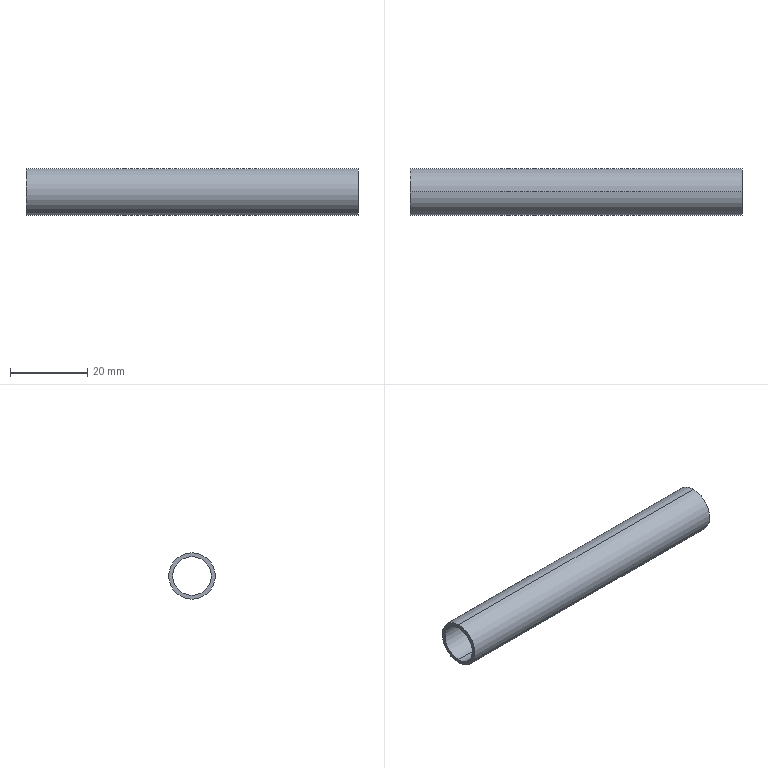Part | SolidWorks | features 3DProfileFeature 2, Sweep 1 | 1 solid | 6 faces | box 85.757 x 12 x 12 mm | volume 2964 mm3 | cylinder 4 | plane 2 | commonest cylinder face diameters 10 x2 12 x2
STEP:
#1=CARTESIAN_POINT('',(860.166,1814.095,417.913));
#2=VERTEX_POINT('',#1);
#3=CARTESIAN_POINT('',(860.166,1814.095,427.913));
#4=VERTEX_POINT('',#3);
#5=CARTESIAN_POINT('',(860.166,1814.095,422.913));
#6=DIRECTION('',(-1.,0.,0.));
#7=DIRECTION('',(0.,0.,1.));
#8=AXIS2_PLACEMENT_3D('',#5,#6,#7);
#9=CIRCLE('',#8,5.);
#10=EDGE_CURVE('',#2,#4,#9,.T.);
#11=ORIENTED_EDGE('',*,*,#10,.F.);
#12=CARTESIAN_POINT('',(774.41,1814.095,417.913));
#13=VERTEX_POINT('',#12);
#14=CARTESIAN_POINT('',(860.166,1814.095,417.913));
#15=DIRECTION('',(-1.,0.,0.));
#16=VECTOR('',#15,1000.);
#17=LINE('',#14,#16);
#18=EDGE_CURVE('',#2,#13,#17,.T.);
#19=ORIENTED_EDGE('',*,*,#18,.T.);
#20=CARTESIAN_POINT('',(774.41,1814.095,427.913));
#21=VERTEX_POINT('',#20);
#22=CARTESIAN_POINT('',(774.41,1814.095,422.913));
#23=DIRECTION('',(-1.,0.,0.));
#24=DIRECTION('',(0.,0.,1.));
#25=AXIS2_PLACEMENT_3D('',#22,#23,#24);
#26=CIRCLE('',#25,5.);
#27=EDGE_CURVE('',#13,#21,#26,.T.);
#28=ORIENTED_EDGE('',*,*,#27,.T.);
#29=CARTESIAN_POINT('',(860.166,1814.095,427.913));
#30=DIRECTION('',(-1.,0.,0.));
#31=VECTOR('',#30,1000.);
#32=LINE('',#29,#31);
#33=EDGE_CURVE('',#4,#21,#32,.T.);
#34=ORIENTED_EDGE('',*,*,#33,.F.);
#35=EDGE_LOOP('',(#11,#19,#28,#34));
#36=FACE_OUTER_BOUND('',#35,.T.);
#37=CARTESIAN_POINT('',(860.166,1814.095,422.913));
#38=DIRECTION('',(-1.,0.,0.));
#39=DIRECTION('',(0.,0.,1.));
#40=AXIS2_PLACEMENT_3D('',#37,#38,#39);
#41=CYLINDRICAL_SURFACE('',#40,5.);
#42=ADVANCED_FACE('',(#36),#41,.F.);
#43=CARTESIAN_POINT('',(860.166,1814.095,428.913));
#44=VERTEX_POINT('',#43);
#45=CARTESIAN_POINT('',(860.166,1814.095,416.913));
#46=VERTEX_POINT('',#45);
#47=CARTESIAN_POINT('',(860.166,1814.095,422.913));
#48=DIRECTION('',(-1.,0.,0.));
#49=DIRECTION('',(0.,0.,1.));
#50=AXIS2_PLACEMENT_3D('',#47,#48,#49);
#51=CIRCLE('',#50,6.);
#52=EDGE_CURVE('',#44,#46,#51,.T.);
#53=ORIENTED_EDGE('',*,*,#52,.T.);
#54=CARTESIAN_POINT('',(774.41,1814.095,416.913));
#55=VERTEX_POINT('',#54);
#56=CARTESIAN_POINT('',(860.166,1814.095,416.913));
#57=DIRECTION('',(-1.,0.,0.));
#58=VECTOR('',#57,1000.);
#59=LINE('',#56,#58);
#60=EDGE_CURVE('',#46,#55,#59,.T.);
#61=ORIENTED_EDGE('',*,*,#60,.T.);
#62=CARTESIAN_POINT('',(774.41,1814.095,428.913));
#63=VERTEX_POINT('',#62);
#64=CARTESIAN_POINT('',(774.41,1814.095,422.913));
#65=DIRECTION('',(-1.,0.,0.));
#66=DIRECTION('',(0.,0.,1.));
#67=AXIS2_PLACEMENT_3D('',#64,#65,#66);
#68=CIRCLE('',#67,6.);
#69=EDGE_CURVE('',#63,#55,#68,.T.);
#70=ORIENTED_EDGE('',*,*,#69,.F.);
#71=CARTESIAN_POINT('',(860.166,1814.095,428.913));
#72=DIRECTION('',(-1.,0.,0.));
#73=VECTOR('',#72,1000.);
#74=LINE('',#71,#73);
#75=EDGE_CURVE('',#44,#63,#74,.T.);
#76=ORIENTED_EDGE('',*,*,#75,.F.);
#77=EDGE_LOOP('',(#53,#61,#70,#76));
#78=FACE_OUTER_BOUND('',#77,.T.);
#79=CARTESIAN_POINT('',(860.166,1814.095,422.913));
#80=DIRECTION('',(-1.,0.,0.));
#81=DIRECTION('',(0.,0.,1.));
#82=AXIS2_PLACEMENT_3D('',#79,#80,#81);
#83=CYLINDRICAL_SURFACE('',#82,6.);
#84=ADVANCED_FACE('',(#78),#83,.T.);
#85=ORIENTED_EDGE('',*,*,#60,.F.);
#86=CARTESIAN_POINT('',(860.166,1814.095,422.913));
#87=DIRECTION('',(-1.,0.,0.));
#88=DIRECTION('',(0.,0.,1.));
#89=AXIS2_PLACEMENT_3D('',#86,#87,#88);
#90=CIRCLE('',#89,6.);
#91=EDGE_CURVE('',#46,#44,#90,.T.);
#92=ORIENTED_EDGE('',*,*,#91,.T.);
#93=ORIENTED_EDGE('',*,*,#75,.T.);
#94=CARTESIAN_POINT('',(774.41,1814.095,422.913));
#95=DIRECTION('',(-1.,0.,0.));
#96=DIRECTION('',(0.,0.,1.));
#97=AXIS2_PLACEMENT_3D('',#94,#95,#96);
#98=CIRCLE('',#97,6.);
#99=EDGE_CURVE('',#55,#63,#98,.T.);
#100=ORIENTED_EDGE('',*,*,#99,.F.);
#101=EDGE_LOOP('',(#85,#92,#93,#100));
#102=FACE_OUTER_BOUND('',#101,.T.);
#103=CARTESIAN_POINT('',(860.166,1814.095,422.913));
#104=DIRECTION('',(-1.,0.,0.));
#105=DIRECTION('',(0.,0.,1.));
#106=AXIS2_PLACEMENT_3D('',#103,#104,#105);
#107=CYLINDRICAL_SURFACE('',#106,6.);
#108=ADVANCED_FACE('',(#102),#107,.T.);
#109=CARTESIAN_POINT('',(774.41,1814.095,422.913));
#110=DIRECTION('',(-1.,0.,0.));
#111=DIRECTION('',(0.,0.,1.));
#112=AXIS2_PLACEMENT_3D('',#109,#110,#111);
#113=CIRCLE('',#112,5.);
#114=EDGE_CURVE('',#21,#13,#113,.T.);
#115=ORIENTED_EDGE('',*,*,#114,.F.);
#116=ORIENTED_EDGE('',*,*,#27,.F.);
#117=EDGE_LOOP('',(#115,#116));
#118=FACE_BOUND('',#117,.T.);
#119=ORIENTED_EDGE('',*,*,#69,.T.);
#120=ORIENTED_EDGE('',*,*,#99,.T.);
#121=EDGE_LOOP('',(#119,#120));
#122=FACE_OUTER_BOUND('',#121,.T.);
#123=CARTESIAN_POINT('',(774.41,1814.095,422.913));
#124=DIRECTION('',(-1.,0.,0.));
#125=DIRECTION('',(0.,0.,1.));
#126=AXIS2_PLACEMENT_3D('',#123,#124,#125);
#127=PLANE('',#126);
#128=ADVANCED_FACE('',(#118,#122),#127,.T.);
#129=CARTESIAN_POINT('',(860.166,1814.095,422.913));
#130=DIRECTION('',(-1.,0.,0.));
#131=DIRECTION('',(0.,0.,1.));
#132=AXIS2_PLACEMENT_3D('',#129,#130,#131);
#133=CIRCLE('',#132,5.);
#134=EDGE_CURVE('',#4,#2,#133,.T.);
#135=ORIENTED_EDGE('',*,*,#134,.T.);
#136=ORIENTED_EDGE('',*,*,#10,.T.);
#137=EDGE_LOOP('',(#135,#136));
#138=FACE_BOUND('',#137,.T.);
#139=ORIENTED_EDGE('',*,*,#52,.F.);
#140=ORIENTED_EDGE('',*,*,#91,.F.);
#141=EDGE_LOOP('',(#139,#140));
#142=FACE_OUTER_BOUND('',#141,.T.);
#143=CARTESIAN_POINT('',(860.166,1814.095,422.913));
#144=DIRECTION('',(-1.,0.,0.));
#145=DIRECTION('',(0.,0.,1.));
#146=AXIS2_PLACEMENT_3D('',#143,#144,#145);
#147=PLANE('',#146);
#148=ADVANCED_FACE('',(#138,#142),#147,.F.);
#149=ORIENTED_EDGE('',*,*,#18,.F.);
#150=ORIENTED_EDGE('',*,*,#134,.F.);
#151=ORIENTED_EDGE('',*,*,#33,.T.);
#152=ORIENTED_EDGE('',*,*,#114,.T.);
#153=EDGE_LOOP('',(#149,#150,#151,#152));
#154=FACE_OUTER_BOUND('',#153,.T.);
#155=CARTESIAN_POINT('',(860.166,1814.095,422.913));
#156=DIRECTION('',(-1.,0.,0.));
#157=DIRECTION('',(0.,0.,1.));
#158=AXIS2_PLACEMENT_3D('',#155,#156,#157);
#159=CYLINDRICAL_SURFACE('',#158,5.);
#160=ADVANCED_FACE('',(#154),#159,.F.);
#161=CLOSED_SHELL('',(#42,#84,#108,#128,#148,#160));
#162=MANIFOLD_SOLID_BREP('',#161);
#163=CARTESIAN_POINT('',(0.,0.,0.));
#164=DIRECTION('',(0.,0.,1.));
#165=DIRECTION('',(1.,0.,0.));
#166=AXIS2_PLACEMENT_3D('',#163,#164,#165);
#167=(LENGTH_UNIT()NAMED_UNIT(*)SI_UNIT(.MILLI.,.METRE.));
#168=UNCERTAINTY_MEASURE_WITH_UNIT(LENGTH_MEASURE(0.00001),#167,'','');
#169=(NAMED_UNIT(*)PLANE_ANGLE_UNIT()SI_UNIT($,.RADIAN.));
#170=(NAMED_UNIT(*)SI_UNIT($,.STERADIAN.)SOLID_ANGLE_UNIT());
#171=(GEOMETRIC_REPRESENTATION_CONTEXT(3)GLOBAL_UNCERTAINTY_ASSIGNED_CONTEXT((#168))GLOBAL_UNIT_ASSIGNED_CONTEXT((#167,#169,#170))REPRESENTATION_CONTEXT('',''));
#172=ADVANCED_BREP_SHAPE_REPRESENTATION('',(#162,#166),#171);